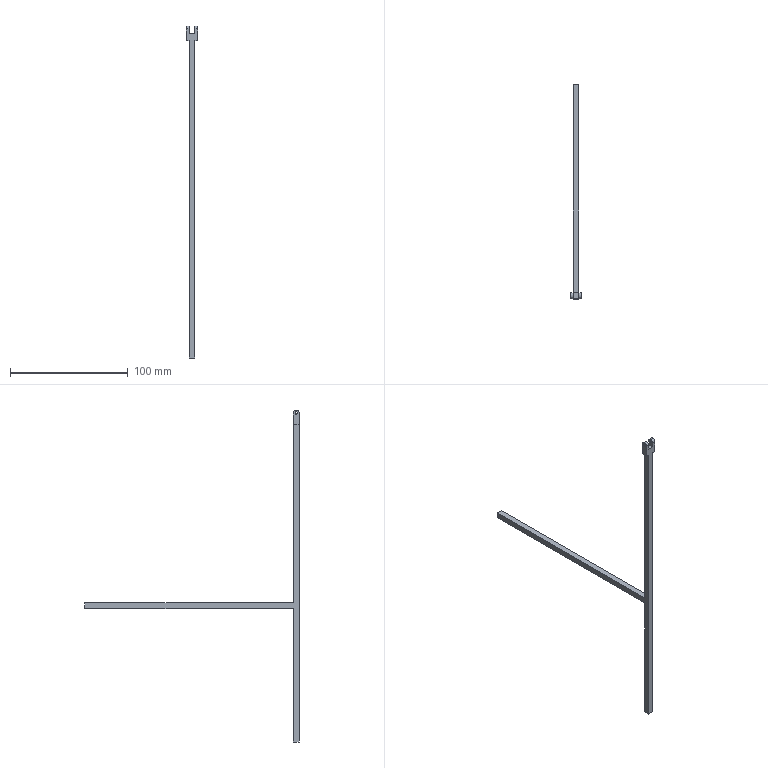Part | SolidWorks | features ICE 4, Extrusion 1 | 1 solid | 22 faces | box 10 x 182.5 x 282.577 mm | volume 11623 mm3 | plane 16 | cylinder 6 | commonest cylinder face diameters 2 x4 5 x2
STEP:
#1=CARTESIAN_POINT('',(2.5,-1.,280.077));
#2=VERTEX_POINT('',#1);
#3=CARTESIAN_POINT('',(2.5,1.,280.077));
#4=VERTEX_POINT('',#3);
#5=CARTESIAN_POINT('',(2.5,0.,280.077));
#6=DIRECTION('',(1.,0.,0.));
#7=DIRECTION('',(0.,1.,0.));
#8=AXIS2_PLACEMENT_3D('',#5,#6,#7);
#9=CIRCLE('',#8,1.);
#10=EDGE_CURVE('',#2,#4,#9,.T.);
#11=ORIENTED_EDGE('',*,*,#10,.F.);
#12=CARTESIAN_POINT('',(5.,-1.,280.077));
#13=VERTEX_POINT('',#12);
#14=CARTESIAN_POINT('',(-5.,-1.,280.077));
#15=DIRECTION('',(1.,0.,0.));
#16=VECTOR('',#15,1000.);
#17=LINE('',#14,#16);
#18=EDGE_CURVE('',#2,#13,#17,.T.);
#19=ORIENTED_EDGE('',*,*,#18,.T.);
#20=CARTESIAN_POINT('',(5.,1.,280.077));
#21=VERTEX_POINT('',#20);
#22=CARTESIAN_POINT('',(5.,0.,280.077));
#23=DIRECTION('',(-1.,0.,0.));
#24=DIRECTION('',(0.,-1.,0.));
#25=AXIS2_PLACEMENT_3D('',#22,#23,#24);
#26=CIRCLE('',#25,1.);
#27=EDGE_CURVE('',#21,#13,#26,.T.);
#28=ORIENTED_EDGE('',*,*,#27,.F.);
#29=CARTESIAN_POINT('',(-5.,1.,280.077));
#30=DIRECTION('',(1.,0.,0.));
#31=VECTOR('',#30,1000.);
#32=LINE('',#29,#31);
#33=EDGE_CURVE('',#4,#21,#32,.T.);
#34=ORIENTED_EDGE('',*,*,#33,.F.);
#35=EDGE_LOOP('',(#11,#19,#28,#34));
#36=FACE_OUTER_BOUND('',#35,.T.);
#37=CARTESIAN_POINT('',(-5.,0.,280.077));
#38=DIRECTION('',(1.,0.,0.));
#39=DIRECTION('',(0.,1.,0.));
#40=AXIS2_PLACEMENT_3D('',#37,#38,#39);
#41=CYLINDRICAL_SURFACE('',#40,1.);
#42=ADVANCED_FACE('',(#36),#41,.F.);
#43=CARTESIAN_POINT('',(-5.,-1.,280.077));
#44=VERTEX_POINT('',#43);
#45=CARTESIAN_POINT('',(-5.,1.,280.077));
#46=VERTEX_POINT('',#45);
#47=CARTESIAN_POINT('',(-5.,0.,280.077));
#48=DIRECTION('',(1.,0.,0.));
#49=DIRECTION('',(0.,1.,0.));
#50=AXIS2_PLACEMENT_3D('',#47,#48,#49);
#51=CIRCLE('',#50,1.);
#52=EDGE_CURVE('',#44,#46,#51,.T.);
#53=ORIENTED_EDGE('',*,*,#52,.F.);
#54=CARTESIAN_POINT('',(-2.5,-1.,280.077));
#55=VERTEX_POINT('',#54);
#56=CARTESIAN_POINT('',(-5.,-1.,280.077));
#57=DIRECTION('',(1.,0.,0.));
#58=VECTOR('',#57,1000.);
#59=LINE('',#56,#58);
#60=EDGE_CURVE('',#44,#55,#59,.T.);
#61=ORIENTED_EDGE('',*,*,#60,.T.);
#62=CARTESIAN_POINT('',(-2.5,1.,280.077));
#63=VERTEX_POINT('',#62);
#64=CARTESIAN_POINT('',(-2.5,0.,280.077));
#65=DIRECTION('',(-1.,0.,0.));
#66=DIRECTION('',(0.,-1.,0.));
#67=AXIS2_PLACEMENT_3D('',#64,#65,#66);
#68=CIRCLE('',#67,1.);
#69=EDGE_CURVE('',#63,#55,#68,.T.);
#70=ORIENTED_EDGE('',*,*,#69,.F.);
#71=CARTESIAN_POINT('',(-5.,1.,280.077));
#72=DIRECTION('',(1.,0.,0.));
#73=VECTOR('',#72,1000.);
#74=LINE('',#71,#73);
#75=EDGE_CURVE('',#46,#63,#74,.T.);
#76=ORIENTED_EDGE('',*,*,#75,.F.);
#77=EDGE_LOOP('',(#53,#61,#70,#76));
#78=FACE_OUTER_BOUND('',#77,.T.);
#79=CARTESIAN_POINT('',(-5.,0.,280.077));
#80=DIRECTION('',(1.,0.,0.));
#81=DIRECTION('',(0.,1.,0.));
#82=AXIS2_PLACEMENT_3D('',#79,#80,#81);
#83=CYLINDRICAL_SURFACE('',#82,1.);
#84=ADVANCED_FACE('',(#78),#83,.F.);
#85=CARTESIAN_POINT('',(2.5,2.5,113.5));
#86=VERTEX_POINT('',#85);
#87=CARTESIAN_POINT('',(-2.5,2.5,113.5));
#88=VERTEX_POINT('',#87);
#89=CARTESIAN_POINT('',(-2.5,2.5,113.5));
#90=DIRECTION('',(-1.,0.,0.));
#91=VECTOR('',#90,1000.);
#92=LINE('',#89,#91);
#93=EDGE_CURVE('',#86,#88,#92,.T.);
#94=ORIENTED_EDGE('',*,*,#93,.F.);
#95=CARTESIAN_POINT('',(2.5,2.5,0.));
#96=VERTEX_POINT('',#95);
#97=CARTESIAN_POINT('',(2.5,2.5,270.));
#98=DIRECTION('',(0.,0.,-1.));
#99=VECTOR('',#98,1000.);
#100=LINE('',#97,#99);
#101=EDGE_CURVE('',#86,#96,#100,.T.);
#102=ORIENTED_EDGE('',*,*,#101,.T.);
#103=CARTESIAN_POINT('',(-2.5,2.5,0.));
#104=VERTEX_POINT('',#103);
#105=CARTESIAN_POINT('',(-2.5,2.5,0.));
#106=DIRECTION('',(-1.,0.,0.));
#107=VECTOR('',#106,1000.);
#108=LINE('',#105,#107);
#109=EDGE_CURVE('',#96,#104,#108,.T.);
#110=ORIENTED_EDGE('',*,*,#109,.T.);
#111=CARTESIAN_POINT('',(-2.5,2.5,270.));
#112=DIRECTION('',(0.,0.,-1.));
#113=VECTOR('',#112,1000.);
#114=LINE('',#111,#113);
#115=EDGE_CURVE('',#88,#104,#114,.T.);
#116=ORIENTED_EDGE('',*,*,#115,.F.);
#117=EDGE_LOOP('',(#94,#102,#110,#116));
#118=FACE_OUTER_BOUND('',#117,.T.);
#119=CARTESIAN_POINT('',(-2.5,2.5,270.));
#120=DIRECTION('',(0.,-1.,0.));
#121=DIRECTION('',(0.,0.,-1.));
#122=AXIS2_PLACEMENT_3D('',#119,#120,#121);
#123=PLANE('',#122);
#124=ADVANCED_FACE('',(#118),#123,.F.);
#125=CARTESIAN_POINT('',(-2.5,2.5,118.5));
#126=VERTEX_POINT('',#125);
#127=CARTESIAN_POINT('',(2.5,2.5,118.5));
#128=VERTEX_POINT('',#127);
#129=CARTESIAN_POINT('',(-2.5,2.5,118.5));
#130=DIRECTION('',(1.,0.,0.));
#131=VECTOR('',#130,1000.);
#132=LINE('',#129,#131);
#133=EDGE_CURVE('',#126,#128,#132,.T.);
#134=ORIENTED_EDGE('',*,*,#133,.F.);
#135=CARTESIAN_POINT('',(-2.5,2.5,270.));
#136=VERTEX_POINT('',#135);
#137=CARTESIAN_POINT('',(-2.5,2.5,270.));
#138=DIRECTION('',(0.,0.,-1.));
#139=VECTOR('',#138,1000.);
#140=LINE('',#137,#139);
#141=EDGE_CURVE('',#136,#126,#140,.T.);
#142=ORIENTED_EDGE('',*,*,#141,.F.);
#143=CARTESIAN_POINT('',(-5.,2.5,270.));
#144=VERTEX_POINT('',#143);
#145=CARTESIAN_POINT('',(-5.,2.5,270.));
#146=DIRECTION('',(-1.,0.,0.));
#147=VECTOR('',#146,1000.);
#148=LINE('',#145,#147);
#149=EDGE_CURVE('',#136,#144,#148,.T.);
#150=ORIENTED_EDGE('',*,*,#149,.T.);
#151=CARTESIAN_POINT('',(-5.,2.5,280.077));
#152=VERTEX_POINT('',#151);
#153=CARTESIAN_POINT('',(-5.,2.5,288.));
#154=DIRECTION('',(0.,0.,-1.));
#155=VECTOR('',#154,1000.);
#156=LINE('',#153,#155);
#157=EDGE_CURVE('',#152,#144,#156,.T.);
#158=ORIENTED_EDGE('',*,*,#157,.F.);
#159=CARTESIAN_POINT('',(-2.5,2.5,280.077));
#160=VERTEX_POINT('',#159);
#161=CARTESIAN_POINT('',(-5.,2.5,280.077));
#162=DIRECTION('',(1.,0.,0.));
#163=VECTOR('',#162,1000.);
#164=LINE('',#161,#163);
#165=EDGE_CURVE('',#152,#160,#164,.T.);
#166=ORIENTED_EDGE('',*,*,#165,.T.);
#167=CARTESIAN_POINT('',(-2.5,2.5,276.));
#168=VERTEX_POINT('',#167);
#169=CARTESIAN_POINT('',(-2.5,2.5,270.));
#170=DIRECTION('',(0.,0.,-1.));
#171=VECTOR('',#170,1000.);
#172=LINE('',#169,#171);
#173=EDGE_CURVE('',#160,#168,#172,.T.);
#174=ORIENTED_EDGE('',*,*,#173,.T.);
#175=CARTESIAN_POINT('',(2.5,2.5,276.));
#176=VERTEX_POINT('',#175);
#177=CARTESIAN_POINT('',(-2.5,2.5,276.));
#178=DIRECTION('',(-1.,0.,0.));
#179=VECTOR('',#178,1000.);
#180=LINE('',#177,#179);
#181=EDGE_CURVE('',#176,#168,#180,.T.);
#182=ORIENTED_EDGE('',*,*,#181,.F.);
#183=CARTESIAN_POINT('',(2.5,2.5,280.077));
#184=VERTEX_POINT('',#183);
#185=CARTESIAN_POINT('',(2.5,2.5,270.));
#186=DIRECTION('',(0.,0.,1.));
#187=VECTOR('',#186,1000.);
#188=LINE('',#185,#187);
#189=EDGE_CURVE('',#176,#184,#188,.T.);
#190=ORIENTED_EDGE('',*,*,#189,.T.);
#191=CARTESIAN_POINT('',(5.,2.5,280.077));
#192=VERTEX_POINT('',#191);
#193=CARTESIAN_POINT('',(-5.,2.5,280.077));
#194=DIRECTION('',(1.,0.,0.));
#195=VECTOR('',#194,1000.);
#196=LINE('',#193,#195);
#197=EDGE_CURVE('',#184,#192,#196,.T.);
#198=ORIENTED_EDGE('',*,*,#197,.T.);
#199=CARTESIAN_POINT('',(5.,2.5,270.));
#200=VERTEX_POINT('',#199);
#201=CARTESIAN_POINT('',(5.,2.5,288.));
#202=DIRECTION('',(0.,0.,-1.));
#203=VECTOR('',#202,1000.);
#204=LINE('',#201,#203);
#205=EDGE_CURVE('',#192,#200,#204,.T.);
#206=ORIENTED_EDGE('',*,*,#205,.T.);
#207=CARTESIAN_POINT('',(2.5,2.5,270.));
#208=VERTEX_POINT('',#207);
#209=CARTESIAN_POINT('',(-5.,2.5,270.));
#210=DIRECTION('',(-1.,0.,0.));
#211=VECTOR('',#210,1000.);
#212=LINE('',#209,#211);
#213=EDGE_CURVE('',#200,#208,#212,.T.);
#214=ORIENTED_EDGE('',*,*,#213,.T.);
#215=CARTESIAN_POINT('',(2.5,2.5,270.));
#216=DIRECTION('',(0.,0.,-1.));
#217=VECTOR('',#216,1000.);
#218=LINE('',#215,#217);
#219=EDGE_CURVE('',#208,#128,#218,.T.);
#220=ORIENTED_EDGE('',*,*,#219,.T.);
#221=EDGE_LOOP('',(#134,#142,#150,#158,#166,#174,#182,#190,#198,#206,#214,#220));
#222=FACE_OUTER_BOUND('',#221,.T.);
#223=CARTESIAN_POINT('',(-2.5,2.5,270.));
#224=DIRECTION('',(0.,-1.,0.));
#225=DIRECTION('',(0.,0.,-1.));
#226=AXIS2_PLACEMENT_3D('',#223,#224,#225);
#227=PLANE('',#226);
#228=ADVANCED_FACE('',(#222),#227,.F.);
#229=ORIENTED_EDGE('',*,*,#101,.F.);
#230=CARTESIAN_POINT('',(2.5,180.,113.5));
#231=VERTEX_POINT('',#230);
#232=CARTESIAN_POINT('',(2.5,180.,113.5));
#233=DIRECTION('',(0.,-1.,0.));
#234=VECTOR('',#233,1000.);
#235=LINE('',#232,#234);
#236=EDGE_CURVE('',#231,#86,#235,.T.);
#237=ORIENTED_EDGE('',*,*,#236,.F.);
#238=CARTESIAN_POINT('',(2.5,180.,118.5));
#239=VERTEX_POINT('',#238);
#240=CARTESIAN_POINT('',(2.5,180.,113.5));
#241=DIRECTION('',(0.,0.,-1.));
#242=VECTOR('',#241,1000.);
#243=LINE('',#240,#242);
#244=EDGE_CURVE('',#239,#231,#243,.T.);
#245=ORIENTED_EDGE('',*,*,#244,.F.);
#246=CARTESIAN_POINT('',(2.5,180.,118.5));
#247=DIRECTION('',(0.,-1.,0.));
#248=VECTOR('',#247,1000.);
#249=LINE('',#246,#248);
#250=EDGE_CURVE('',#239,#128,#249,.T.);
#251=ORIENTED_EDGE('',*,*,#250,.T.);
#252=ORIENTED_EDGE('',*,*,#219,.F.);
#253=CARTESIAN_POINT('',(2.5,-2.5,270.));
#254=VERTEX_POINT('',#253);
#255=CARTESIAN_POINT('',(2.5,2.5,270.));
#256=DIRECTION('',(0.,1.,0.));
#257=VECTOR('',#256,1000.);
#258=LINE('',#255,#257);
#259=EDGE_CURVE('',#254,#208,#258,.T.);
#260=ORIENTED_EDGE('',*,*,#259,.F.);
#261=CARTESIAN_POINT('',(2.5,-2.5,0.));
#262=VERTEX_POINT('',#261);
#263=CARTESIAN_POINT('',(2.5,-2.5,270.));
#264=DIRECTION('',(0.,0.,-1.));
#265=VECTOR('',#264,1000.);
#266=LINE('',#263,#265);
#267=EDGE_CURVE('',#254,#262,#266,.T.);
#268=ORIENTED_EDGE('',*,*,#267,.T.);
#269=CARTESIAN_POINT('',(2.5,2.5,0.));
#270=DIRECTION('',(0.,1.,0.));
#271=VECTOR('',#270,1000.);
#272=LINE('',#269,#271);
#273=EDGE_CURVE('',#262,#96,#272,.T.);
#274=ORIENTED_EDGE('',*,*,#273,.T.);
#275=EDGE_LOOP('',(#229,#237,#245,#251,#252,#260,#268,#274));
#276=FACE_OUTER_BOUND('',#275,.T.);
#277=CARTESIAN_POINT('',(2.5,2.5,270.));
#278=DIRECTION('',(-1.,0.,0.));
#279=DIRECTION('',(0.,-1.,0.));
#280=AXIS2_PLACEMENT_3D('',#277,#278,#279);
#281=PLANE('',#280);
#282=ADVANCED_FACE('',(#276),#281,.F.);
#283=ORIENTED_EDGE('',*,*,#141,.T.);
#284=CARTESIAN_POINT('',(-2.5,180.,118.5));
#285=VERTEX_POINT('',#284);
#286=CARTESIAN_POINT('',(-2.5,180.,118.5));
#287=DIRECTION('',(0.,-1.,0.));
#288=VECTOR('',#287,1000.);
#289=LINE('',#286,#288);
#290=EDGE_CURVE('',#285,#126,#289,.T.);
#291=ORIENTED_EDGE('',*,*,#290,.F.);
#292=CARTESIAN_POINT('',(-2.5,180.,113.5));
#293=VERTEX_POINT('',#292);
#294=CARTESIAN_POINT('',(-2.5,180.,113.5));
#295=DIRECTION('',(0.,0.,1.));
#296=VECTOR('',#295,1000.);
#297=LINE('',#294,#296);
#298=EDGE_CURVE('',#293,#285,#297,.T.);
#299=ORIENTED_EDGE('',*,*,#298,.F.);
#300=CARTESIAN_POINT('',(-2.5,180.,113.5));
#301=DIRECTION('',(0.,-1.,0.));
#302=VECTOR('',#301,1000.);
#303=LINE('',#300,#302);
#304=EDGE_CURVE('',#293,#88,#303,.T.);
#305=ORIENTED_EDGE('',*,*,#304,.T.);
#306=ORIENTED_EDGE('',*,*,#115,.T.);
#307=CARTESIAN_POINT('',(-2.5,-2.5,0.));
#308=VERTEX_POINT('',#307);
#309=CARTESIAN_POINT('',(-2.5,2.5,0.));
#310=DIRECTION('',(0.,-1.,0.));
#311=VECTOR('',#310,1000.);
#312=LINE('',#309,#311);
#313=EDGE_CURVE('',#104,#308,#312,.T.);
#314=ORIENTED_EDGE('',*,*,#313,.T.);
#315=CARTESIAN_POINT('',(-2.5,-2.5,270.));
#316=VERTEX_POINT('',#315);
#317=CARTESIAN_POINT('',(-2.5,-2.5,270.));
#318=DIRECTION('',(0.,0.,-1.));
#319=VECTOR('',#318,1000.);
#320=LINE('',#317,#319);
#321=EDGE_CURVE('',#316,#308,#320,.T.);
#322=ORIENTED_EDGE('',*,*,#321,.F.);
#323=CARTESIAN_POINT('',(-2.5,2.5,270.));
#324=DIRECTION('',(0.,-1.,0.));
#325=VECTOR('',#324,1000.);
#326=LINE('',#323,#325);
#327=EDGE_CURVE('',#136,#316,#326,.T.);
#328=ORIENTED_EDGE('',*,*,#327,.F.);
#329=EDGE_LOOP('',(#283,#291,#299,#305,#306,#314,#322,#328));
#330=FACE_OUTER_BOUND('',#329,.T.);
#331=CARTESIAN_POINT('',(-2.5,2.5,270.));
#332=DIRECTION('',(1.,0.,0.));
#333=DIRECTION('',(0.,1.,0.));
#334=AXIS2_PLACEMENT_3D('',#331,#332,#333);
#335=PLANE('',#334);
#336=ADVANCED_FACE('',(#330),#335,.F.);
#337=CARTESIAN_POINT('',(5.,-2.5,280.077));
#338=VERTEX_POINT('',#337);
#339=CARTESIAN_POINT('',(5.,-2.5,270.));
#340=VERTEX_POINT('',#339);
#341=CARTESIAN_POINT('',(5.,-2.5,288.));
#342=DIRECTION('',(0.,0.,-1.));
#343=VECTOR('',#342,1000.);
#344=LINE('',#341,#343);
#345=EDGE_CURVE('',#338,#340,#344,.T.);
#346=ORIENTED_EDGE('',*,*,#345,.F.);
#347=CARTESIAN_POINT('',(2.5,-2.5,280.077));
#348=VERTEX_POINT('',#347);
#349=CARTESIAN_POINT('',(-5.,-2.5,280.077));
#350=DIRECTION('',(1.,0.,0.));
#351=VECTOR('',#350,1000.);
#352=LINE('',#349,#351);
#353=EDGE_CURVE('',#348,#338,#352,.T.);
#354=ORIENTED_EDGE('',*,*,#353,.F.);
#355=CARTESIAN_POINT('',(2.5,-2.5,276.));
#356=VERTEX_POINT('',#355);
#357=CARTESIAN_POINT('',(2.5,-2.5,270.));
#358=DIRECTION('',(0.,0.,-1.));
#359=VECTOR('',#358,1000.);
#360=LINE('',#357,#359);
#361=EDGE_CURVE('',#348,#356,#360,.T.);
#362=ORIENTED_EDGE('',*,*,#361,.T.);
#363=CARTESIAN_POINT('',(-2.5,-2.5,276.));
#364=VERTEX_POINT('',#363);
#365=CARTESIAN_POINT('',(-2.5,-2.5,276.));
#366=DIRECTION('',(1.,0.,0.));
#367=VECTOR('',#366,1000.);
#368=LINE('',#365,#367);
#369=EDGE_CURVE('',#364,#356,#368,.T.);
#370=ORIENTED_EDGE('',*,*,#369,.F.);
#371=CARTESIAN_POINT('',(-2.5,-2.5,280.077));
#372=VERTEX_POINT('',#371);
#373=CARTESIAN_POINT('',(-2.5,-2.5,270.));
#374=DIRECTION('',(0.,0.,1.));
#375=VECTOR('',#374,1000.);
#376=LINE('',#373,#375);
#377=EDGE_CURVE('',#364,#372,#376,.T.);
#378=ORIENTED_EDGE('',*,*,#377,.T.);
#379=CARTESIAN_POINT('',(-5.,-2.5,280.077));
#380=VERTEX_POINT('',#379);
#381=CARTESIAN_POINT('',(-5.,-2.5,280.077));
#382=DIRECTION('',(1.,0.,0.));
#383=VECTOR('',#382,1000.);
#384=LINE('',#381,#383);
#385=EDGE_CURVE('',#380,#372,#384,.T.);
#386=ORIENTED_EDGE('',*,*,#385,.F.);
#387=CARTESIAN_POINT('',(-5.,-2.5,270.));
#388=VERTEX_POINT('',#387);
#389=CARTESIAN_POINT('',(-5.,-2.5,288.));
#390=DIRECTION('',(0.,0.,-1.));
#391=VECTOR('',#390,1000.);
#392=LINE('',#389,#391);
#393=EDGE_CURVE('',#380,#388,#392,.T.);
#394=ORIENTED_EDGE('',*,*,#393,.T.);
#395=CARTESIAN_POINT('',(-5.,-2.5,270.));
#396=DIRECTION('',(1.,0.,0.));
#397=VECTOR('',#396,1000.);
#398=LINE('',#395,#397);
#399=EDGE_CURVE('',#388,#316,#398,.T.);
#400=ORIENTED_EDGE('',*,*,#399,.T.);
#401=ORIENTED_EDGE('',*,*,#321,.T.);
#402=CARTESIAN_POINT('',(-2.5,-2.5,0.));
#403=DIRECTION('',(1.,0.,0.));
#404=VECTOR('',#403,1000.);
#405=LINE('',#402,#404);
#406=EDGE_CURVE('',#308,#262,#405,.T.);
#407=ORIENTED_EDGE('',*,*,#406,.T.);
#408=ORIENTED_EDGE('',*,*,#267,.F.);
#409=CARTESIAN_POINT('',(-5.,-2.5,270.));
#410=DIRECTION('',(1.,0.,0.));
#411=VECTOR('',#410,1000.);
#412=LINE('',#409,#411);
#413=EDGE_CURVE('',#254,#340,#412,.T.);
#414=ORIENTED_EDGE('',*,*,#413,.T.);
#415=EDGE_LOOP('',(#346,#354,#362,#370,#378,#386,#394,#400,#401,#407,#408,#414));
#416=FACE_OUTER_BOUND('',#415,.T.);
#417=CARTESIAN_POINT('',(-2.5,-2.5,270.));
#418=DIRECTION('',(0.,1.,0.));
#419=DIRECTION('',(0.,0.,1.));
#420=AXIS2_PLACEMENT_3D('',#417,#418,#419);
#421=PLANE('',#420);
#422=ADVANCED_FACE('',(#416),#421,.F.);
#423=ORIENTED_EDGE('',*,*,#273,.F.);
#424=ORIENTED_EDGE('',*,*,#406,.F.);
#425=ORIENTED_EDGE('',*,*,#313,.F.);
#426=ORIENTED_EDGE('',*,*,#109,.F.);
#427=EDGE_LOOP('',(#423,#424,#425,#426));
#428=FACE_OUTER_BOUND('',#427,.T.);
#429=CARTESIAN_POINT('',(0.,0.,0.));
#430=DIRECTION('',(0.,0.,1.));
#431=DIRECTION('',(1.,0.,0.));
#432=AXIS2_PLACEMENT_3D('',#429,#430,#431);
#433=PLANE('',#432);
#434=ADVANCED_FACE('',(#428),#433,.F.);
#435=ORIENTED_EDGE('',*,*,#413,.F.);
#436=ORIENTED_EDGE('',*,*,#259,.T.);
#437=ORIENTED_EDGE('',*,*,#213,.F.);
#438=CARTESIAN_POINT('',(5.,2.5,270.));
#439=DIRECTION('',(0.,1.,0.));
#440=VECTOR('',#439,1000.);
#441=LINE('',#438,#440);
#442=EDGE_CURVE('',#340,#200,#441,.T.);
#443=ORIENTED_EDGE('',*,*,#442,.F.);
#444=EDGE_LOOP('',(#435,#436,#437,#443));
#445=FACE_OUTER_BOUND('',#444,.T.);
#446=CARTESIAN_POINT('',(0.,0.,270.));
#447=DIRECTION('',(0.,0.,1.));
#448=DIRECTION('',(1.,0.,0.));
#449=AXIS2_PLACEMENT_3D('',#446,#447,#448);
#450=PLANE('',#449);
#451=ADVANCED_FACE('',(#445),#450,.F.);
#452=ORIENTED_EDGE('',*,*,#149,.F.);
#453=ORIENTED_EDGE('',*,*,#327,.T.);
#454=ORIENTED_EDGE('',*,*,#399,.F.);
#455=CARTESIAN_POINT('',(-5.,2.5,270.));
#456=DIRECTION('',(0.,-1.,0.));
#457=VECTOR('',#456,1000.);
#458=LINE('',#455,#457);
#459=EDGE_CURVE('',#144,#388,#458,.T.);
#460=ORIENTED_EDGE('',*,*,#459,.F.);
#461=EDGE_LOOP('',(#452,#453,#454,#460));
#462=FACE_OUTER_BOUND('',#461,.T.);
#463=CARTESIAN_POINT('',(0.,0.,270.));
#464=DIRECTION('',(0.,0.,1.));
#465=DIRECTION('',(1.,0.,0.));
#466=AXIS2_PLACEMENT_3D('',#463,#464,#465);
#467=PLANE('',#466);
#468=ADVANCED_FACE('',(#462),#467,.F.);
#469=ORIENTED_EDGE('',*,*,#27,.T.);
#470=CARTESIAN_POINT('',(5.,0.,280.077));
#471=DIRECTION('',(-1.,0.,0.));
#472=DIRECTION('',(0.,-1.,0.));
#473=AXIS2_PLACEMENT_3D('',#470,#471,#472);
#474=CIRCLE('',#473,1.);
#475=EDGE_CURVE('',#13,#21,#474,.T.);
#476=ORIENTED_EDGE('',*,*,#475,.T.);
#477=EDGE_LOOP('',(#469,#476));
#478=FACE_BOUND('',#477,.T.);
#479=ORIENTED_EDGE('',*,*,#205,.F.);
#480=CARTESIAN_POINT('',(5.,0.,280.077));
#481=DIRECTION('',(-1.,0.,0.));
#482=DIRECTION('',(0.,1.,0.));
#483=AXIS2_PLACEMENT_3D('',#480,#481,#482);
#484=CIRCLE('',#483,2.5);
#485=EDGE_CURVE('',#338,#192,#484,.T.);
#486=ORIENTED_EDGE('',*,*,#485,.F.);
#487=ORIENTED_EDGE('',*,*,#345,.T.);
#488=ORIENTED_EDGE('',*,*,#442,.T.);
#489=EDGE_LOOP('',(#479,#486,#487,#488));
#490=FACE_OUTER_BOUND('',#489,.T.);
#491=CARTESIAN_POINT('',(5.,2.5,288.));
#492=DIRECTION('',(-1.,0.,0.));
#493=DIRECTION('',(0.,-1.,0.));
#494=AXIS2_PLACEMENT_3D('',#491,#492,#493);
#495=PLANE('',#494);
#496=ADVANCED_FACE('',(#478,#490),#495,.F.);
#497=CARTESIAN_POINT('',(-5.,0.,280.077));
#498=DIRECTION('',(1.,0.,0.));
#499=DIRECTION('',(0.,1.,0.));
#500=AXIS2_PLACEMENT_3D('',#497,#498,#499);
#501=CIRCLE('',#500,1.);
#502=EDGE_CURVE('',#46,#44,#501,.T.);
#503=ORIENTED_EDGE('',*,*,#502,.T.);
#504=ORIENTED_EDGE('',*,*,#52,.T.);
#505=EDGE_LOOP('',(#503,#504));
#506=FACE_BOUND('',#505,.T.);
#507=ORIENTED_EDGE('',*,*,#393,.F.);
#508=CARTESIAN_POINT('',(-5.,0.,280.077));
#509=DIRECTION('',(-1.,0.,0.));
#510=DIRECTION('',(0.,1.,0.));
#511=AXIS2_PLACEMENT_3D('',#508,#509,#510);
#512=CIRCLE('',#511,2.5);
#513=EDGE_CURVE('',#380,#152,#512,.T.);
#514=ORIENTED_EDGE('',*,*,#513,.T.);
#515=ORIENTED_EDGE('',*,*,#157,.T.);
#516=ORIENTED_EDGE('',*,*,#459,.T.);
#517=EDGE_LOOP('',(#507,#514,#515,#516));
#518=FACE_OUTER_BOUND('',#517,.T.);
#519=CARTESIAN_POINT('',(-5.,2.5,288.));
#520=DIRECTION('',(1.,0.,0.));
#521=DIRECTION('',(0.,0.,-1.));
#522=AXIS2_PLACEMENT_3D('',#519,#520,#521);
#523=PLANE('',#522);
#524=ADVANCED_FACE('',(#506,#518),#523,.F.);
#525=ORIENTED_EDGE('',*,*,#181,.T.);
#526=CARTESIAN_POINT('',(-2.5,9.679,276.));
#527=DIRECTION('',(0.,-1.,0.));
#528=VECTOR('',#527,1000.);
#529=LINE('',#526,#528);
#530=EDGE_CURVE('',#168,#364,#529,.T.);
#531=ORIENTED_EDGE('',*,*,#530,.T.);
#532=ORIENTED_EDGE('',*,*,#369,.T.);
#533=CARTESIAN_POINT('',(2.5,9.679,276.));
#534=DIRECTION('',(0.,1.,0.));
#535=VECTOR('',#534,1000.);
#536=LINE('',#533,#535);
#537=EDGE_CURVE('',#356,#176,#536,.T.);
#538=ORIENTED_EDGE('',*,*,#537,.T.);
#539=EDGE_LOOP('',(#525,#531,#532,#538));
#540=FACE_OUTER_BOUND('',#539,.T.);
#541=CARTESIAN_POINT('',(0.,0.,276.));
#542=DIRECTION('',(0.,0.,1.));
#543=DIRECTION('',(1.,0.,0.));
#544=AXIS2_PLACEMENT_3D('',#541,#542,#543);
#545=PLANE('',#544);
#546=ADVANCED_FACE('',(#540),#545,.T.);
#547=CARTESIAN_POINT('',(2.5,0.,280.077));
#548=DIRECTION('',(1.,0.,0.));
#549=DIRECTION('',(0.,1.,0.));
#550=AXIS2_PLACEMENT_3D('',#547,#548,#549);
#551=CIRCLE('',#550,1.);
#552=EDGE_CURVE('',#4,#2,#551,.T.);
#553=ORIENTED_EDGE('',*,*,#552,.T.);
#554=ORIENTED_EDGE('',*,*,#10,.T.);
#555=EDGE_LOOP('',(#553,#554));
#556=FACE_BOUND('',#555,.T.);
#557=ORIENTED_EDGE('',*,*,#361,.F.);
#558=CARTESIAN_POINT('',(2.5,0.,280.077));
#559=DIRECTION('',(-1.,0.,0.));
#560=DIRECTION('',(0.,1.,0.));
#561=AXIS2_PLACEMENT_3D('',#558,#559,#560);
#562=CIRCLE('',#561,2.5);
#563=EDGE_CURVE('',#348,#184,#562,.T.);
#564=ORIENTED_EDGE('',*,*,#563,.T.);
#565=ORIENTED_EDGE('',*,*,#189,.F.);
#566=ORIENTED_EDGE('',*,*,#537,.F.);
#567=EDGE_LOOP('',(#557,#564,#565,#566));
#568=FACE_OUTER_BOUND('',#567,.T.);
#569=CARTESIAN_POINT('',(2.5,9.679,276.));
#570=DIRECTION('',(1.,0.,0.));
#571=DIRECTION('',(0.,1.,0.));
#572=AXIS2_PLACEMENT_3D('',#569,#570,#571);
#573=PLANE('',#572);
#574=ADVANCED_FACE('',(#556,#568),#573,.F.);
#575=ORIENTED_EDGE('',*,*,#69,.T.);
#576=CARTESIAN_POINT('',(-2.5,0.,280.077));
#577=DIRECTION('',(-1.,0.,0.));
#578=DIRECTION('',(0.,-1.,0.));
#579=AXIS2_PLACEMENT_3D('',#576,#577,#578);
#580=CIRCLE('',#579,1.);
#581=EDGE_CURVE('',#55,#63,#580,.T.);
#582=ORIENTED_EDGE('',*,*,#581,.T.);
#583=EDGE_LOOP('',(#575,#582));
#584=FACE_BOUND('',#583,.T.);
#585=ORIENTED_EDGE('',*,*,#173,.F.);
#586=CARTESIAN_POINT('',(-2.5,0.,280.077));
#587=DIRECTION('',(1.,0.,0.));
#588=DIRECTION('',(0.,-1.,0.));
#589=AXIS2_PLACEMENT_3D('',#586,#587,#588);
#590=CIRCLE('',#589,2.5);
#591=EDGE_CURVE('',#160,#372,#590,.T.);
#592=ORIENTED_EDGE('',*,*,#591,.T.);
#593=ORIENTED_EDGE('',*,*,#377,.F.);
#594=ORIENTED_EDGE('',*,*,#530,.F.);
#595=EDGE_LOOP('',(#585,#592,#593,#594));
#596=FACE_OUTER_BOUND('',#595,.T.);
#597=CARTESIAN_POINT('',(-2.5,9.679,276.));
#598=DIRECTION('',(-1.,0.,0.));
#599=DIRECTION('',(0.,-1.,0.));
#600=AXIS2_PLACEMENT_3D('',#597,#598,#599);
#601=PLANE('',#600);
#602=ADVANCED_FACE('',(#584,#596),#601,.F.);
#603=ORIENTED_EDGE('',*,*,#60,.F.);
#604=ORIENTED_EDGE('',*,*,#502,.F.);
#605=ORIENTED_EDGE('',*,*,#75,.T.);
#606=ORIENTED_EDGE('',*,*,#581,.F.);
#607=EDGE_LOOP('',(#603,#604,#605,#606));
#608=FACE_OUTER_BOUND('',#607,.T.);
#609=CARTESIAN_POINT('',(-5.,0.,280.077));
#610=DIRECTION('',(1.,0.,0.));
#611=DIRECTION('',(0.,1.,0.));
#612=AXIS2_PLACEMENT_3D('',#609,#610,#611);
#613=CYLINDRICAL_SURFACE('',#612,1.);
#614=ADVANCED_FACE('',(#608),#613,.F.);
#615=ORIENTED_EDGE('',*,*,#165,.F.);
#616=ORIENTED_EDGE('',*,*,#513,.F.);
#617=ORIENTED_EDGE('',*,*,#385,.T.);
#618=ORIENTED_EDGE('',*,*,#591,.F.);
#619=EDGE_LOOP('',(#615,#616,#617,#618));
#620=FACE_OUTER_BOUND('',#619,.T.);
#621=CARTESIAN_POINT('',(-5.,0.,280.077));
#622=DIRECTION('',(1.,0.,0.));
#623=DIRECTION('',(0.,1.,0.));
#624=AXIS2_PLACEMENT_3D('',#621,#622,#623);
#625=CYLINDRICAL_SURFACE('',#624,2.5);
#626=ADVANCED_FACE('',(#620),#625,.T.);
#627=ORIENTED_EDGE('',*,*,#18,.F.);
#628=ORIENTED_EDGE('',*,*,#552,.F.);
#629=ORIENTED_EDGE('',*,*,#33,.T.);
#630=ORIENTED_EDGE('',*,*,#475,.F.);
#631=EDGE_LOOP('',(#627,#628,#629,#630));
#632=FACE_OUTER_BOUND('',#631,.T.);
#633=CARTESIAN_POINT('',(-5.,0.,280.077));
#634=DIRECTION('',(1.,0.,0.));
#635=DIRECTION('',(0.,1.,0.));
#636=AXIS2_PLACEMENT_3D('',#633,#634,#635);
#637=CYLINDRICAL_SURFACE('',#636,1.);
#638=ADVANCED_FACE('',(#632),#637,.F.);
#639=ORIENTED_EDGE('',*,*,#197,.F.);
#640=ORIENTED_EDGE('',*,*,#563,.F.);
#641=ORIENTED_EDGE('',*,*,#353,.T.);
#642=ORIENTED_EDGE('',*,*,#485,.T.);
#643=EDGE_LOOP('',(#639,#640,#641,#642));
#644=FACE_OUTER_BOUND('',#643,.T.);
#645=CARTESIAN_POINT('',(-5.,0.,280.077));
#646=DIRECTION('',(1.,0.,0.));
#647=DIRECTION('',(0.,1.,0.));
#648=AXIS2_PLACEMENT_3D('',#645,#646,#647);
#649=CYLINDRICAL_SURFACE('',#648,2.5);
#650=ADVANCED_FACE('',(#644),#649,.T.);
#651=ORIENTED_EDGE('',*,*,#236,.T.);
#652=ORIENTED_EDGE('',*,*,#93,.T.);
#653=ORIENTED_EDGE('',*,*,#304,.F.);
#654=CARTESIAN_POINT('',(-2.5,180.,113.5));
#655=DIRECTION('',(-1.,0.,0.));
#656=VECTOR('',#655,1000.);
#657=LINE('',#654,#656);
#658=EDGE_CURVE('',#231,#293,#657,.T.);
#659=ORIENTED_EDGE('',*,*,#658,.F.);
#660=EDGE_LOOP('',(#651,#652,#653,#659));
#661=FACE_OUTER_BOUND('',#660,.T.);
#662=CARTESIAN_POINT('',(-2.5,180.,113.5));
#663=DIRECTION('',(0.,0.,1.));
#664=DIRECTION('',(1.,0.,0.));
#665=AXIS2_PLACEMENT_3D('',#662,#663,#664);
#666=PLANE('',#665);
#667=ADVANCED_FACE('',(#661),#666,.F.);
#668=ORIENTED_EDGE('',*,*,#290,.T.);
#669=ORIENTED_EDGE('',*,*,#133,.T.);
#670=ORIENTED_EDGE('',*,*,#250,.F.);
#671=CARTESIAN_POINT('',(-2.5,180.,118.5));
#672=DIRECTION('',(1.,0.,0.));
#673=VECTOR('',#672,1000.);
#674=LINE('',#671,#673);
#675=EDGE_CURVE('',#285,#239,#674,.T.);
#676=ORIENTED_EDGE('',*,*,#675,.F.);
#677=EDGE_LOOP('',(#668,#669,#670,#676));
#678=FACE_OUTER_BOUND('',#677,.T.);
#679=CARTESIAN_POINT('',(-2.5,180.,118.5));
#680=DIRECTION('',(0.,0.,-1.));
#681=DIRECTION('',(-1.,0.,0.));
#682=AXIS2_PLACEMENT_3D('',#679,#680,#681);
#683=PLANE('',#682);
#684=ADVANCED_FACE('',(#678),#683,.F.);
#685=ORIENTED_EDGE('',*,*,#244,.T.);
#686=ORIENTED_EDGE('',*,*,#658,.T.);
#687=ORIENTED_EDGE('',*,*,#298,.T.);
#688=ORIENTED_EDGE('',*,*,#675,.T.);
#689=EDGE_LOOP('',(#685,#686,#687,#688));
#690=FACE_OUTER_BOUND('',#689,.T.);
#691=CARTESIAN_POINT('',(0.,180.,0.));
#692=DIRECTION('',(0.,1.,0.));
#693=DIRECTION('',(0.,0.,1.));
#694=AXIS2_PLACEMENT_3D('',#691,#692,#693);
#695=PLANE('',#694);
#696=ADVANCED_FACE('',(#690),#695,.T.);
#697=CLOSED_SHELL('',(#42,#84,#124,#228,#282,#336,#422,#434,#451,#468,#496,#524,#546,#574,#602,#614,#626,#638,#650,#667,#684,#696));
#698=MANIFOLD_SOLID_BREP('',#697);
#699=CARTESIAN_POINT('',(0.,0.,0.));
#700=DIRECTION('',(0.,0.,1.));
#701=DIRECTION('',(1.,0.,0.));
#702=AXIS2_PLACEMENT_3D('',#699,#700,#701);
#703=(LENGTH_UNIT()NAMED_UNIT(*)SI_UNIT(.MILLI.,.METRE.));
#704=UNCERTAINTY_MEASURE_WITH_UNIT(LENGTH_MEASURE(0.00001),#703,'','');
#705=(NAMED_UNIT(*)PLANE_ANGLE_UNIT()SI_UNIT($,.RADIAN.));
#706=(NAMED_UNIT(*)SI_UNIT($,.STERADIAN.)SOLID_ANGLE_UNIT());
#707=(GEOMETRIC_REPRESENTATION_CONTEXT(3)GLOBAL_UNCERTAINTY_ASSIGNED_CONTEXT((#704))GLOBAL_UNIT_ASSIGNED_CONTEXT((#703,#705,#706))REPRESENTATION_CONTEXT('',''));
#708=ADVANCED_BREP_SHAPE_REPRESENTATION('',(#698,#702),#707);